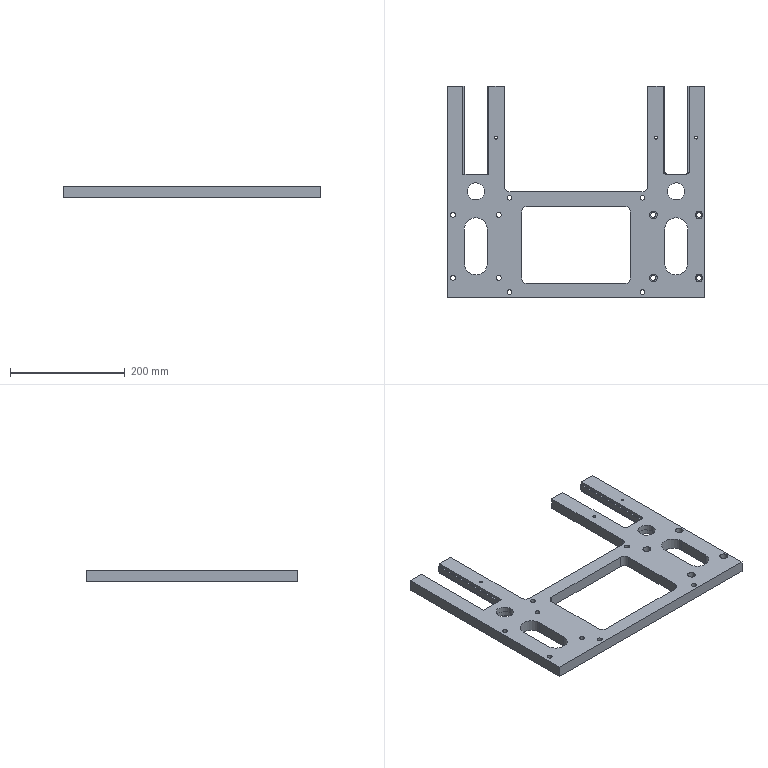Part | STEP file | A14-011 | 1 solid | 110 faces | box 450 x 370 x 20 mm | volume 1435092 mm3 | cylinder 62 | plane 48 | commonest cylinder face diameters 8.5 x24 13.5 x8 5 x6 10 x6 20 x6 30 x4